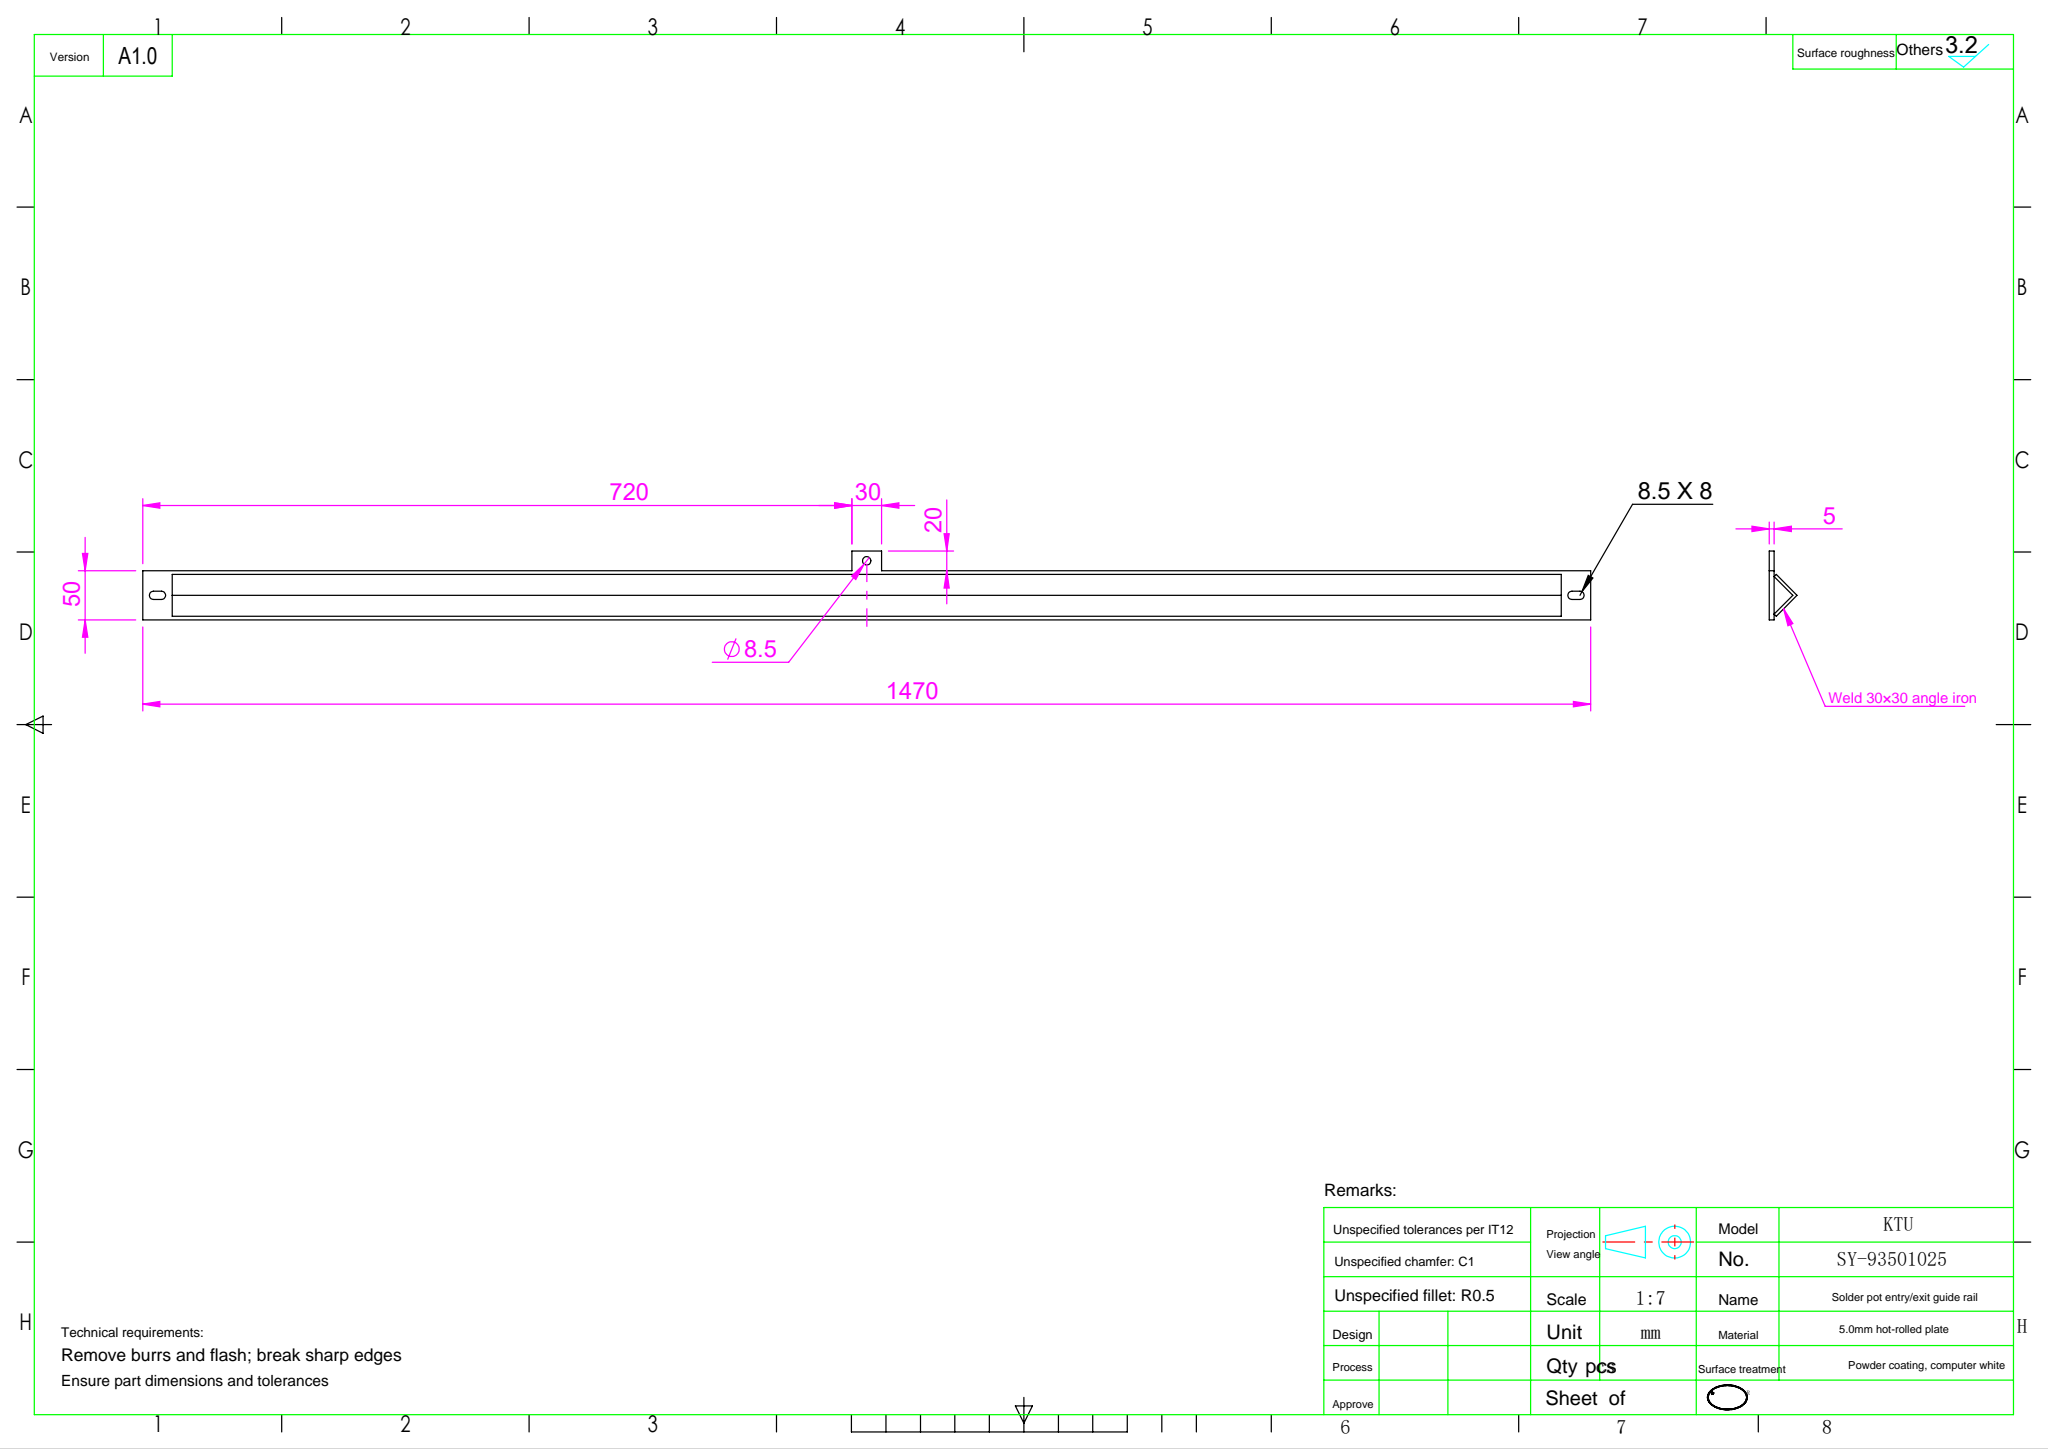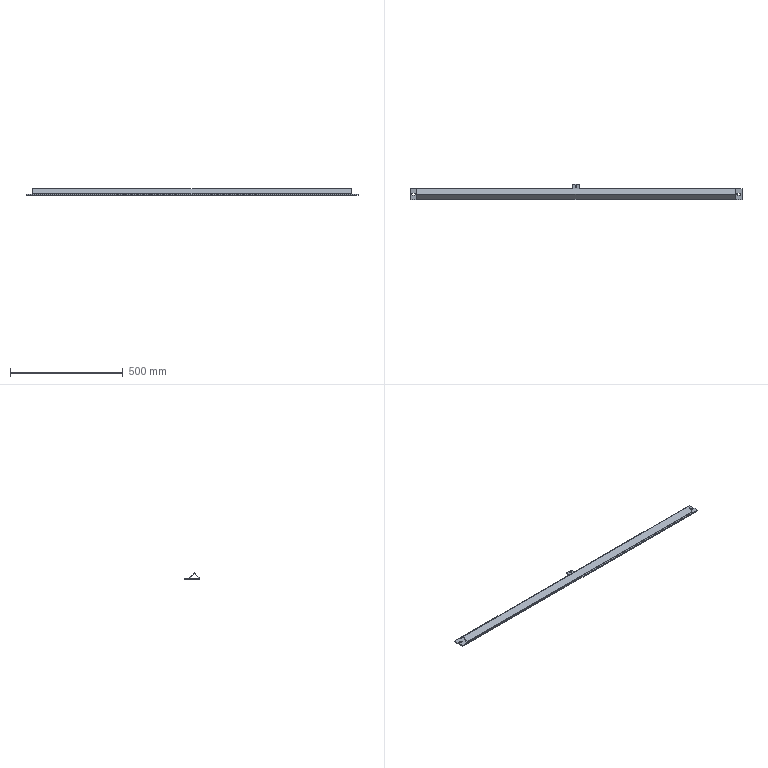Part | SolidWorks | features ICE 4, Extrusion 1 | 2 solids | 30 faces | box 1470 x 70 x 28.335 mm | volume 610079 mm3 | plane 22 | cylinder 8 | commonest cylinder face diameters 8.5 x8
STEP:
#1=CARTESIAN_POINT('',(-705.,21.213,4.621));
#2=VERTEX_POINT('',#1);
#3=CARTESIAN_POINT('',(-705.,19.092,2.5));
#4=VERTEX_POINT('',#3);
#5=CARTESIAN_POINT('',(-705.,21.213,4.621));
#6=DIRECTION('',(0.,-0.7071,-0.7071));
#7=VECTOR('',#6,1000.);
#8=LINE('',#5,#7);
#9=EDGE_CURVE('',#2,#4,#8,.T.);
#10=ORIENTED_EDGE('',*,*,#9,.F.);
#11=CARTESIAN_POINT('',(705.,21.213,4.621));
#12=VERTEX_POINT('',#11);
#13=CARTESIAN_POINT('',(705.,21.213,4.621));
#14=DIRECTION('',(-1.,0.,0.));
#15=VECTOR('',#14,1000.);
#16=LINE('',#13,#15);
#17=EDGE_CURVE('',#12,#2,#16,.T.);
#18=ORIENTED_EDGE('',*,*,#17,.F.);
#19=CARTESIAN_POINT('',(705.,19.092,2.5));
#20=VERTEX_POINT('',#19);
#21=CARTESIAN_POINT('',(705.,21.213,4.621));
#22=DIRECTION('',(0.,-0.7071,-0.7071));
#23=VECTOR('',#22,1000.);
#24=LINE('',#21,#23);
#25=EDGE_CURVE('',#12,#20,#24,.T.);
#26=ORIENTED_EDGE('',*,*,#25,.T.);
#27=CARTESIAN_POINT('',(705.,19.092,2.5));
#28=DIRECTION('',(-1.,0.,0.));
#29=VECTOR('',#28,1000.);
#30=LINE('',#27,#29);
#31=EDGE_CURVE('',#20,#4,#30,.T.);
#32=ORIENTED_EDGE('',*,*,#31,.T.);
#33=EDGE_LOOP('',(#10,#18,#26,#32));
#34=FACE_OUTER_BOUND('',#33,.T.);
#35=CARTESIAN_POINT('',(705.,21.213,4.621));
#36=DIRECTION('',(0.,0.7071,-0.7071));
#37=DIRECTION('',(0.,0.7071,0.7071));
#38=AXIS2_PLACEMENT_3D('',#35,#36,#37);
#39=PLANE('',#38);
#40=ADVANCED_FACE('',(#34),#39,.T.);
#41=CARTESIAN_POINT('',(-705.,0.,25.835));
#42=VERTEX_POINT('',#41);
#43=CARTESIAN_POINT('',(-705.,21.213,4.621));
#44=DIRECTION('',(0.,0.7071,-0.7071));
#45=VECTOR('',#44,1000.);
#46=LINE('',#43,#45);
#47=EDGE_CURVE('',#42,#2,#46,.T.);
#48=ORIENTED_EDGE('',*,*,#47,.F.);
#49=CARTESIAN_POINT('',(705.,0.,25.835));
#50=VERTEX_POINT('',#49);
#51=CARTESIAN_POINT('',(705.,0.,25.835));
#52=DIRECTION('',(-1.,0.,0.));
#53=VECTOR('',#52,1000.);
#54=LINE('',#51,#53);
#55=EDGE_CURVE('',#50,#42,#54,.T.);
#56=ORIENTED_EDGE('',*,*,#55,.F.);
#57=CARTESIAN_POINT('',(705.,21.213,4.621));
#58=DIRECTION('',(0.,0.7071,-0.7071));
#59=VECTOR('',#58,1000.);
#60=LINE('',#57,#59);
#61=EDGE_CURVE('',#50,#12,#60,.T.);
#62=ORIENTED_EDGE('',*,*,#61,.T.);
#63=ORIENTED_EDGE('',*,*,#17,.T.);
#64=EDGE_LOOP('',(#48,#56,#62,#63));
#65=FACE_OUTER_BOUND('',#64,.T.);
#66=CARTESIAN_POINT('',(705.,21.213,4.621));
#67=DIRECTION('',(0.,0.7071,0.7071));
#68=DIRECTION('',(0.,-0.7071,0.7071));
#69=AXIS2_PLACEMENT_3D('',#66,#67,#68);
#70=PLANE('',#69);
#71=ADVANCED_FACE('',(#65),#70,.T.);
#72=CARTESIAN_POINT('',(-705.,-21.213,4.621));
#73=VERTEX_POINT('',#72);
#74=CARTESIAN_POINT('',(-705.,0.,25.835));
#75=DIRECTION('',(0.,0.7071,0.7071));
#76=VECTOR('',#75,1000.);
#77=LINE('',#74,#76);
#78=EDGE_CURVE('',#73,#42,#77,.T.);
#79=ORIENTED_EDGE('',*,*,#78,.F.);
#80=CARTESIAN_POINT('',(705.,-21.213,4.621));
#81=VERTEX_POINT('',#80);
#82=CARTESIAN_POINT('',(705.,-21.213,4.621));
#83=DIRECTION('',(-1.,0.,0.));
#84=VECTOR('',#83,1000.);
#85=LINE('',#82,#84);
#86=EDGE_CURVE('',#81,#73,#85,.T.);
#87=ORIENTED_EDGE('',*,*,#86,.F.);
#88=CARTESIAN_POINT('',(705.,0.,25.835));
#89=DIRECTION('',(0.,0.7071,0.7071));
#90=VECTOR('',#89,1000.);
#91=LINE('',#88,#90);
#92=EDGE_CURVE('',#81,#50,#91,.T.);
#93=ORIENTED_EDGE('',*,*,#92,.T.);
#94=ORIENTED_EDGE('',*,*,#55,.T.);
#95=EDGE_LOOP('',(#79,#87,#93,#94));
#96=FACE_OUTER_BOUND('',#95,.T.);
#97=CARTESIAN_POINT('',(705.,0.,25.835));
#98=DIRECTION('',(0.,-0.7071,0.7071));
#99=DIRECTION('',(0.,-0.7071,-0.7071));
#100=AXIS2_PLACEMENT_3D('',#97,#98,#99);
#101=PLANE('',#100);
#102=ADVANCED_FACE('',(#96),#101,.T.);
#103=CARTESIAN_POINT('',(-705.,-19.092,2.5));
#104=VERTEX_POINT('',#103);
#105=CARTESIAN_POINT('',(-705.,-19.092,2.5));
#106=DIRECTION('',(0.,-0.7071,0.7071));
#107=VECTOR('',#106,1000.);
#108=LINE('',#105,#107);
#109=EDGE_CURVE('',#104,#73,#108,.T.);
#110=ORIENTED_EDGE('',*,*,#109,.F.);
#111=CARTESIAN_POINT('',(705.,-19.092,2.5));
#112=VERTEX_POINT('',#111);
#113=CARTESIAN_POINT('',(705.,-19.092,2.5));
#114=DIRECTION('',(-1.,0.,0.));
#115=VECTOR('',#114,1000.);
#116=LINE('',#113,#115);
#117=EDGE_CURVE('',#112,#104,#116,.T.);
#118=ORIENTED_EDGE('',*,*,#117,.F.);
#119=CARTESIAN_POINT('',(705.,-19.092,2.5));
#120=DIRECTION('',(0.,-0.7071,0.7071));
#121=VECTOR('',#120,1000.);
#122=LINE('',#119,#121);
#123=EDGE_CURVE('',#112,#81,#122,.T.);
#124=ORIENTED_EDGE('',*,*,#123,.T.);
#125=ORIENTED_EDGE('',*,*,#86,.T.);
#126=EDGE_LOOP('',(#110,#118,#124,#125));
#127=FACE_OUTER_BOUND('',#126,.T.);
#128=CARTESIAN_POINT('',(705.,-19.092,2.5));
#129=DIRECTION('',(0.,-0.7071,-0.7071));
#130=DIRECTION('',(0.,0.7071,-0.7071));
#131=AXIS2_PLACEMENT_3D('',#128,#129,#130);
#132=PLANE('',#131);
#133=ADVANCED_FACE('',(#127),#132,.T.);
#134=CARTESIAN_POINT('',(-705.,0.,21.592));
#135=VERTEX_POINT('',#134);
#136=CARTESIAN_POINT('',(-705.,0.,21.592));
#137=DIRECTION('',(0.,-0.7071,-0.7071));
#138=VECTOR('',#137,1000.);
#139=LINE('',#136,#138);
#140=EDGE_CURVE('',#135,#104,#139,.T.);
#141=ORIENTED_EDGE('',*,*,#140,.F.);
#142=CARTESIAN_POINT('',(705.,0.,21.592));
#143=VERTEX_POINT('',#142);
#144=CARTESIAN_POINT('',(705.,0.,21.592));
#145=DIRECTION('',(-1.,0.,0.));
#146=VECTOR('',#145,1000.);
#147=LINE('',#144,#146);
#148=EDGE_CURVE('',#143,#135,#147,.T.);
#149=ORIENTED_EDGE('',*,*,#148,.F.);
#150=CARTESIAN_POINT('',(705.,0.,21.592));
#151=DIRECTION('',(0.,-0.7071,-0.7071));
#152=VECTOR('',#151,1000.);
#153=LINE('',#150,#152);
#154=EDGE_CURVE('',#143,#112,#153,.T.);
#155=ORIENTED_EDGE('',*,*,#154,.T.);
#156=ORIENTED_EDGE('',*,*,#117,.T.);
#157=EDGE_LOOP('',(#141,#149,#155,#156));
#158=FACE_OUTER_BOUND('',#157,.T.);
#159=CARTESIAN_POINT('',(705.,0.,21.592));
#160=DIRECTION('',(0.,0.7071,-0.7071));
#161=DIRECTION('',(0.,0.7071,0.7071));
#162=AXIS2_PLACEMENT_3D('',#159,#160,#161);
#163=PLANE('',#162);
#164=ADVANCED_FACE('',(#158),#163,.T.);
#165=CARTESIAN_POINT('',(-705.,19.092,2.5));
#166=DIRECTION('',(0.,-0.7071,0.7071));
#167=VECTOR('',#166,1000.);
#168=LINE('',#165,#167);
#169=EDGE_CURVE('',#4,#135,#168,.T.);
#170=ORIENTED_EDGE('',*,*,#169,.F.);
#171=ORIENTED_EDGE('',*,*,#31,.F.);
#172=CARTESIAN_POINT('',(705.,19.092,2.5));
#173=DIRECTION('',(0.,-0.7071,0.7071));
#174=VECTOR('',#173,1000.);
#175=LINE('',#172,#174);
#176=EDGE_CURVE('',#20,#143,#175,.T.);
#177=ORIENTED_EDGE('',*,*,#176,.T.);
#178=ORIENTED_EDGE('',*,*,#148,.T.);
#179=EDGE_LOOP('',(#170,#171,#177,#178));
#180=FACE_OUTER_BOUND('',#179,.T.);
#181=CARTESIAN_POINT('',(705.,19.092,2.5));
#182=DIRECTION('',(0.,-0.7071,-0.7071));
#183=DIRECTION('',(0.,0.7071,-0.7071));
#184=AXIS2_PLACEMENT_3D('',#181,#182,#183);
#185=PLANE('',#184);
#186=ADVANCED_FACE('',(#180),#185,.T.);
#187=ORIENTED_EDGE('',*,*,#25,.F.);
#188=ORIENTED_EDGE('',*,*,#61,.F.);
#189=ORIENTED_EDGE('',*,*,#92,.F.);
#190=ORIENTED_EDGE('',*,*,#123,.F.);
#191=ORIENTED_EDGE('',*,*,#154,.F.);
#192=ORIENTED_EDGE('',*,*,#176,.F.);
#193=EDGE_LOOP('',(#187,#188,#189,#190,#191,#192));
#194=FACE_OUTER_BOUND('',#193,.T.);
#195=CARTESIAN_POINT('',(705.,0.,0.));
#196=DIRECTION('',(-1.,0.,0.));
#197=DIRECTION('',(0.,0.,1.));
#198=AXIS2_PLACEMENT_3D('',#195,#196,#197);
#199=PLANE('',#198);
#200=ADVANCED_FACE('',(#194),#199,.F.);
#201=ORIENTED_EDGE('',*,*,#9,.T.);
#202=ORIENTED_EDGE('',*,*,#169,.T.);
#203=ORIENTED_EDGE('',*,*,#140,.T.);
#204=ORIENTED_EDGE('',*,*,#109,.T.);
#205=ORIENTED_EDGE('',*,*,#78,.T.);
#206=ORIENTED_EDGE('',*,*,#47,.T.);
#207=EDGE_LOOP('',(#201,#202,#203,#204,#205,#206));
#208=FACE_OUTER_BOUND('',#207,.T.);
#209=CARTESIAN_POINT('',(-705.,0.,0.));
#210=DIRECTION('',(-1.,0.,0.));
#211=DIRECTION('',(0.,0.,1.));
#212=AXIS2_PLACEMENT_3D('',#209,#210,#211);
#213=PLANE('',#212);
#214=ADVANCED_FACE('',(#208),#213,.T.);
#215=CLOSED_SHELL('',(#40,#71,#102,#133,#164,#186,#200,#214));
#216=MANIFOLD_SOLID_BREP('',#215);
#217=CARTESIAN_POINT('',(4.25,35.,-2.5));
#218=VERTEX_POINT('',#217);
#219=CARTESIAN_POINT('',(-4.25,35.,-2.5));
#220=VERTEX_POINT('',#219);
#221=CARTESIAN_POINT('',(0.,35.,-2.5));
#222=DIRECTION('',(0.,0.,-1.));
#223=DIRECTION('',(1.,0.,0.));
#224=AXIS2_PLACEMENT_3D('',#221,#222,#223);
#225=CIRCLE('',#224,4.25);
#226=EDGE_CURVE('',#218,#220,#225,.T.);
#227=ORIENTED_EDGE('',*,*,#226,.T.);
#228=CARTESIAN_POINT('',(-4.25,35.,2.5));
#229=VERTEX_POINT('',#228);
#230=CARTESIAN_POINT('',(-4.25,35.,-2.501));
#231=DIRECTION('',(0.,0.,1.));
#232=VECTOR('',#231,1000.);
#233=LINE('',#230,#232);
#234=EDGE_CURVE('',#220,#229,#233,.T.);
#235=ORIENTED_EDGE('',*,*,#234,.T.);
#236=CARTESIAN_POINT('',(4.25,35.,2.5));
#237=VERTEX_POINT('',#236);
#238=CARTESIAN_POINT('',(0.,35.,2.5));
#239=DIRECTION('',(0.,0.,1.));
#240=DIRECTION('',(1.,0.,0.));
#241=AXIS2_PLACEMENT_3D('',#238,#239,#240);
#242=CIRCLE('',#241,4.25);
#243=EDGE_CURVE('',#229,#237,#242,.T.);
#244=ORIENTED_EDGE('',*,*,#243,.T.);
#245=CARTESIAN_POINT('',(4.25,35.,-2.501));
#246=DIRECTION('',(0.,0.,1.));
#247=VECTOR('',#246,1000.);
#248=LINE('',#245,#247);
#249=EDGE_CURVE('',#218,#237,#248,.T.);
#250=ORIENTED_EDGE('',*,*,#249,.F.);
#251=EDGE_LOOP('',(#227,#235,#244,#250));
#252=FACE_OUTER_BOUND('',#251,.T.);
#253=CARTESIAN_POINT('',(0.,35.,-2.501));
#254=DIRECTION('',(0.,0.,1.));
#255=DIRECTION('',(1.,0.,0.));
#256=AXIS2_PLACEMENT_3D('',#253,#254,#255);
#257=CYLINDRICAL_SURFACE('',#256,4.25);
#258=ADVANCED_FACE('',(#252),#257,.F.);
#259=CARTESIAN_POINT('',(-716.,4.25,-2.5));
#260=VERTEX_POINT('',#259);
#261=CARTESIAN_POINT('',(-711.75,0.,-2.5));
#262=VERTEX_POINT('',#261);
#263=CARTESIAN_POINT('',(-716.,0.,-2.5));
#264=DIRECTION('',(0.,0.,-1.));
#265=DIRECTION('',(1.,0.,0.));
#266=AXIS2_PLACEMENT_3D('',#263,#264,#265);
#267=CIRCLE('',#266,4.25);
#268=EDGE_CURVE('',#260,#262,#267,.T.);
#269=ORIENTED_EDGE('',*,*,#268,.T.);
#270=CARTESIAN_POINT('',(-711.75,0.,2.5));
#271=VERTEX_POINT('',#270);
#272=CARTESIAN_POINT('',(-711.75,0.,-2.501));
#273=DIRECTION('',(0.,0.,1.));
#274=VECTOR('',#273,1000.);
#275=LINE('',#272,#274);
#276=EDGE_CURVE('',#262,#271,#275,.T.);
#277=ORIENTED_EDGE('',*,*,#276,.T.);
#278=CARTESIAN_POINT('',(-716.,4.25,2.5));
#279=VERTEX_POINT('',#278);
#280=CARTESIAN_POINT('',(-716.,0.,2.5));
#281=DIRECTION('',(0.,0.,1.));
#282=DIRECTION('',(1.,0.,0.));
#283=AXIS2_PLACEMENT_3D('',#280,#281,#282);
#284=CIRCLE('',#283,4.25);
#285=EDGE_CURVE('',#271,#279,#284,.T.);
#286=ORIENTED_EDGE('',*,*,#285,.T.);
#287=CARTESIAN_POINT('',(-716.,4.25,-2.501));
#288=DIRECTION('',(0.,0.,1.));
#289=VECTOR('',#288,1000.);
#290=LINE('',#287,#289);
#291=EDGE_CURVE('',#260,#279,#290,.T.);
#292=ORIENTED_EDGE('',*,*,#291,.F.);
#293=EDGE_LOOP('',(#269,#277,#286,#292));
#294=FACE_OUTER_BOUND('',#293,.T.);
#295=CARTESIAN_POINT('',(-716.,0.,-2.501));
#296=DIRECTION('',(0.,0.,1.));
#297=DIRECTION('',(1.,0.,0.));
#298=AXIS2_PLACEMENT_3D('',#295,#296,#297);
#299=CYLINDRICAL_SURFACE('',#298,4.25);
#300=ADVANCED_FACE('',(#294),#299,.F.);
#301=CARTESIAN_POINT('',(724.,4.25,-2.5));
#302=VERTEX_POINT('',#301);
#303=CARTESIAN_POINT('',(728.25,0.,-2.5));
#304=VERTEX_POINT('',#303);
#305=CARTESIAN_POINT('',(724.,0.,-2.5));
#306=DIRECTION('',(0.,0.,-1.));
#307=DIRECTION('',(1.,0.,0.));
#308=AXIS2_PLACEMENT_3D('',#305,#306,#307);
#309=CIRCLE('',#308,4.25);
#310=EDGE_CURVE('',#302,#304,#309,.T.);
#311=ORIENTED_EDGE('',*,*,#310,.T.);
#312=CARTESIAN_POINT('',(728.25,0.,2.5));
#313=VERTEX_POINT('',#312);
#314=CARTESIAN_POINT('',(728.25,0.,-2.501));
#315=DIRECTION('',(0.,0.,1.));
#316=VECTOR('',#315,1000.);
#317=LINE('',#314,#316);
#318=EDGE_CURVE('',#304,#313,#317,.T.);
#319=ORIENTED_EDGE('',*,*,#318,.T.);
#320=CARTESIAN_POINT('',(724.,4.25,2.5));
#321=VERTEX_POINT('',#320);
#322=CARTESIAN_POINT('',(724.,0.,2.5));
#323=DIRECTION('',(0.,0.,1.));
#324=DIRECTION('',(1.,0.,0.));
#325=AXIS2_PLACEMENT_3D('',#322,#323,#324);
#326=CIRCLE('',#325,4.25);
#327=EDGE_CURVE('',#313,#321,#326,.T.);
#328=ORIENTED_EDGE('',*,*,#327,.T.);
#329=CARTESIAN_POINT('',(724.,4.25,-2.501));
#330=DIRECTION('',(0.,0.,1.));
#331=VECTOR('',#330,1000.);
#332=LINE('',#329,#331);
#333=EDGE_CURVE('',#302,#321,#332,.T.);
#334=ORIENTED_EDGE('',*,*,#333,.F.);
#335=EDGE_LOOP('',(#311,#319,#328,#334));
#336=FACE_OUTER_BOUND('',#335,.T.);
#337=CARTESIAN_POINT('',(724.,0.,-2.501));
#338=DIRECTION('',(0.,0.,1.));
#339=DIRECTION('',(1.,0.,0.));
#340=AXIS2_PLACEMENT_3D('',#337,#338,#339);
#341=CYLINDRICAL_SURFACE('',#340,4.25);
#342=ADVANCED_FACE('',(#336),#341,.F.);
#343=CARTESIAN_POINT('',(-15.,25.,-2.5));
#344=VERTEX_POINT('',#343);
#345=CARTESIAN_POINT('',(-15.,25.,2.5));
#346=VERTEX_POINT('',#345);
#347=CARTESIAN_POINT('',(-15.,25.,-2.5));
#348=DIRECTION('',(0.,0.,1.));
#349=VECTOR('',#348,1000.);
#350=LINE('',#347,#349);
#351=EDGE_CURVE('',#344,#346,#350,.T.);
#352=ORIENTED_EDGE('',*,*,#351,.F.);
#353=CARTESIAN_POINT('',(-735.,25.,-2.5));
#354=VERTEX_POINT('',#353);
#355=CARTESIAN_POINT('',(-735.,25.,-2.5));
#356=DIRECTION('',(-1.,0.,0.));
#357=VECTOR('',#356,1000.);
#358=LINE('',#355,#357);
#359=EDGE_CURVE('',#344,#354,#358,.T.);
#360=ORIENTED_EDGE('',*,*,#359,.T.);
#361=CARTESIAN_POINT('',(-735.,25.,2.5));
#362=VERTEX_POINT('',#361);
#363=CARTESIAN_POINT('',(-735.,25.,2.5));
#364=DIRECTION('',(0.,0.,-1.));
#365=VECTOR('',#364,1000.);
#366=LINE('',#363,#365);
#367=EDGE_CURVE('',#362,#354,#366,.T.);
#368=ORIENTED_EDGE('',*,*,#367,.F.);
#369=CARTESIAN_POINT('',(-735.,25.,2.5));
#370=DIRECTION('',(-1.,0.,0.));
#371=VECTOR('',#370,1000.);
#372=LINE('',#369,#371);
#373=EDGE_CURVE('',#346,#362,#372,.T.);
#374=ORIENTED_EDGE('',*,*,#373,.F.);
#375=EDGE_LOOP('',(#352,#360,#368,#374));
#376=FACE_OUTER_BOUND('',#375,.T.);
#377=CARTESIAN_POINT('',(-735.,25.,2.5));
#378=DIRECTION('',(0.,-1.,0.));
#379=DIRECTION('',(0.,0.,-1.));
#380=AXIS2_PLACEMENT_3D('',#377,#378,#379);
#381=PLANE('',#380);
#382=ADVANCED_FACE('',(#376),#381,.F.);
#383=CARTESIAN_POINT('',(735.,-25.,-2.5));
#384=VERTEX_POINT('',#383);
#385=CARTESIAN_POINT('',(735.,25.,-2.5));
#386=VERTEX_POINT('',#385);
#387=CARTESIAN_POINT('',(735.,25.,-2.5));
#388=DIRECTION('',(0.,1.,0.));
#389=VECTOR('',#388,1000.);
#390=LINE('',#387,#389);
#391=EDGE_CURVE('',#384,#386,#390,.T.);
#392=ORIENTED_EDGE('',*,*,#391,.T.);
#393=CARTESIAN_POINT('',(735.,25.,2.5));
#394=VERTEX_POINT('',#393);
#395=CARTESIAN_POINT('',(735.,25.,2.5));
#396=DIRECTION('',(0.,0.,-1.));
#397=VECTOR('',#396,1000.);
#398=LINE('',#395,#397);
#399=EDGE_CURVE('',#394,#386,#398,.T.);
#400=ORIENTED_EDGE('',*,*,#399,.F.);
#401=CARTESIAN_POINT('',(735.,-25.,2.5));
#402=VERTEX_POINT('',#401);
#403=CARTESIAN_POINT('',(735.,25.,2.5));
#404=DIRECTION('',(0.,1.,0.));
#405=VECTOR('',#404,1000.);
#406=LINE('',#403,#405);
#407=EDGE_CURVE('',#402,#394,#406,.T.);
#408=ORIENTED_EDGE('',*,*,#407,.F.);
#409=CARTESIAN_POINT('',(735.,-25.,2.5));
#410=DIRECTION('',(0.,0.,-1.));
#411=VECTOR('',#410,1000.);
#412=LINE('',#409,#411);
#413=EDGE_CURVE('',#402,#384,#412,.T.);
#414=ORIENTED_EDGE('',*,*,#413,.T.);
#415=EDGE_LOOP('',(#392,#400,#408,#414));
#416=FACE_OUTER_BOUND('',#415,.T.);
#417=CARTESIAN_POINT('',(735.,25.,2.5));
#418=DIRECTION('',(-1.,0.,0.));
#419=DIRECTION('',(0.,0.,1.));
#420=AXIS2_PLACEMENT_3D('',#417,#418,#419);
#421=PLANE('',#420);
#422=ADVANCED_FACE('',(#416),#421,.F.);
#423=CARTESIAN_POINT('',(15.,25.,-2.5));
#424=VERTEX_POINT('',#423);
#425=CARTESIAN_POINT('',(-735.,25.,-2.5));
#426=DIRECTION('',(-1.,0.,0.));
#427=VECTOR('',#426,1000.);
#428=LINE('',#425,#427);
#429=EDGE_CURVE('',#386,#424,#428,.T.);
#430=ORIENTED_EDGE('',*,*,#429,.T.);
#431=CARTESIAN_POINT('',(15.,25.,2.5));
#432=VERTEX_POINT('',#431);
#433=CARTESIAN_POINT('',(15.,25.,-2.5));
#434=DIRECTION('',(0.,0.,1.));
#435=VECTOR('',#434,1000.);
#436=LINE('',#433,#435);
#437=EDGE_CURVE('',#424,#432,#436,.T.);
#438=ORIENTED_EDGE('',*,*,#437,.T.);
#439=CARTESIAN_POINT('',(-735.,25.,2.5));
#440=DIRECTION('',(-1.,0.,0.));
#441=VECTOR('',#440,1000.);
#442=LINE('',#439,#441);
#443=EDGE_CURVE('',#394,#432,#442,.T.);
#444=ORIENTED_EDGE('',*,*,#443,.F.);
#445=ORIENTED_EDGE('',*,*,#399,.T.);
#446=EDGE_LOOP('',(#430,#438,#444,#445));
#447=FACE_OUTER_BOUND('',#446,.T.);
#448=CARTESIAN_POINT('',(-735.,25.,2.5));
#449=DIRECTION('',(0.,-1.,0.));
#450=DIRECTION('',(0.,0.,-1.));
#451=AXIS2_PLACEMENT_3D('',#448,#449,#450);
#452=PLANE('',#451);
#453=ADVANCED_FACE('',(#447),#452,.F.);
#454=CARTESIAN_POINT('',(-735.,-25.,-2.5));
#455=VERTEX_POINT('',#454);
#456=CARTESIAN_POINT('',(-735.,25.,-2.5));
#457=DIRECTION('',(0.,-1.,0.));
#458=VECTOR('',#457,1000.);
#459=LINE('',#456,#458);
#460=EDGE_CURVE('',#354,#455,#459,.T.);
#461=ORIENTED_EDGE('',*,*,#460,.T.);
#462=CARTESIAN_POINT('',(-735.,-25.,2.5));
#463=VERTEX_POINT('',#462);
#464=CARTESIAN_POINT('',(-735.,-25.,2.5));
#465=DIRECTION('',(0.,0.,-1.));
#466=VECTOR('',#465,1000.);
#467=LINE('',#464,#466);
#468=EDGE_CURVE('',#463,#455,#467,.T.);
#469=ORIENTED_EDGE('',*,*,#468,.F.);
#470=CARTESIAN_POINT('',(-735.,25.,2.5));
#471=DIRECTION('',(0.,-1.,0.));
#472=VECTOR('',#471,1000.);
#473=LINE('',#470,#472);
#474=EDGE_CURVE('',#362,#463,#473,.T.);
#475=ORIENTED_EDGE('',*,*,#474,.F.);
#476=ORIENTED_EDGE('',*,*,#367,.T.);
#477=EDGE_LOOP('',(#461,#469,#475,#476));
#478=FACE_OUTER_BOUND('',#477,.T.);
#479=CARTESIAN_POINT('',(-735.,25.,2.5));
#480=DIRECTION('',(1.,0.,0.));
#481=DIRECTION('',(0.,0.,-1.));
#482=AXIS2_PLACEMENT_3D('',#479,#480,#481);
#483=PLANE('',#482);
#484=ADVANCED_FACE('',(#478),#483,.F.);
#485=CARTESIAN_POINT('',(-735.,-25.,-2.5));
#486=DIRECTION('',(1.,0.,0.));
#487=VECTOR('',#486,1000.);
#488=LINE('',#485,#487);
#489=EDGE_CURVE('',#455,#384,#488,.T.);
#490=ORIENTED_EDGE('',*,*,#489,.T.);
#491=ORIENTED_EDGE('',*,*,#413,.F.);
#492=CARTESIAN_POINT('',(-735.,-25.,2.5));
#493=DIRECTION('',(1.,0.,0.));
#494=VECTOR('',#493,1000.);
#495=LINE('',#492,#494);
#496=EDGE_CURVE('',#463,#402,#495,.T.);
#497=ORIENTED_EDGE('',*,*,#496,.F.);
#498=ORIENTED_EDGE('',*,*,#468,.T.);
#499=EDGE_LOOP('',(#490,#491,#497,#498));
#500=FACE_OUTER_BOUND('',#499,.T.);
#501=CARTESIAN_POINT('',(-735.,-25.,2.5));
#502=DIRECTION('',(0.,1.,0.));
#503=DIRECTION('',(0.,0.,1.));
#504=AXIS2_PLACEMENT_3D('',#501,#502,#503);
#505=PLANE('',#504);
#506=ADVANCED_FACE('',(#500),#505,.F.);
#507=CARTESIAN_POINT('',(0.,35.,2.5));
#508=DIRECTION('',(0.,0.,1.));
#509=DIRECTION('',(1.,0.,0.));
#510=AXIS2_PLACEMENT_3D('',#507,#508,#509);
#511=CIRCLE('',#510,4.25);
#512=EDGE_CURVE('',#237,#229,#511,.T.);
#513=ORIENTED_EDGE('',*,*,#512,.F.);
#514=ORIENTED_EDGE('',*,*,#243,.F.);
#515=EDGE_LOOP('',(#513,#514));
#516=FACE_BOUND('',#515,.T.);
#517=CARTESIAN_POINT('',(-716.,-4.25,2.5));
#518=VERTEX_POINT('',#517);
#519=CARTESIAN_POINT('',(-716.,0.,2.5));
#520=DIRECTION('',(0.,0.,1.));
#521=DIRECTION('',(1.,0.,0.));
#522=AXIS2_PLACEMENT_3D('',#519,#520,#521);
#523=CIRCLE('',#522,4.25);
#524=EDGE_CURVE('',#518,#271,#523,.T.);
#525=ORIENTED_EDGE('',*,*,#524,.F.);
#526=CARTESIAN_POINT('',(-724.,-4.25,2.5));
#527=VERTEX_POINT('',#526);
#528=CARTESIAN_POINT('',(-716.,-4.25,2.5));
#529=DIRECTION('',(1.,0.,0.));
#530=VECTOR('',#529,1000.);
#531=LINE('',#528,#530);
#532=EDGE_CURVE('',#527,#518,#531,.T.);
#533=ORIENTED_EDGE('',*,*,#532,.F.);
#534=CARTESIAN_POINT('',(-724.,4.25,2.5));
#535=VERTEX_POINT('',#534);
#536=CARTESIAN_POINT('',(-724.,0.,2.5));
#537=DIRECTION('',(0.,0.,1.));
#538=DIRECTION('',(1.,0.,0.));
#539=AXIS2_PLACEMENT_3D('',#536,#537,#538);
#540=CIRCLE('',#539,4.25);
#541=EDGE_CURVE('',#535,#527,#540,.T.);
#542=ORIENTED_EDGE('',*,*,#541,.F.);
#543=CARTESIAN_POINT('',(-716.,4.25,2.5));
#544=DIRECTION('',(-1.,0.,0.));
#545=VECTOR('',#544,1000.);
#546=LINE('',#543,#545);
#547=EDGE_CURVE('',#279,#535,#546,.T.);
#548=ORIENTED_EDGE('',*,*,#547,.F.);
#549=ORIENTED_EDGE('',*,*,#285,.F.);
#550=EDGE_LOOP('',(#525,#533,#542,#548,#549));
#551=FACE_BOUND('',#550,.T.);
#552=CARTESIAN_POINT('',(716.,4.25,2.5));
#553=VERTEX_POINT('',#552);
#554=CARTESIAN_POINT('',(716.,-4.25,2.5));
#555=VERTEX_POINT('',#554);
#556=CARTESIAN_POINT('',(716.,0.,2.5));
#557=DIRECTION('',(0.,0.,1.));
#558=DIRECTION('',(1.,0.,0.));
#559=AXIS2_PLACEMENT_3D('',#556,#557,#558);
#560=CIRCLE('',#559,4.25);
#561=EDGE_CURVE('',#553,#555,#560,.T.);
#562=ORIENTED_EDGE('',*,*,#561,.F.);
#563=CARTESIAN_POINT('',(716.,4.25,2.5));
#564=DIRECTION('',(-1.,0.,0.));
#565=VECTOR('',#564,1000.);
#566=LINE('',#563,#565);
#567=EDGE_CURVE('',#321,#553,#566,.T.);
#568=ORIENTED_EDGE('',*,*,#567,.F.);
#569=ORIENTED_EDGE('',*,*,#327,.F.);
#570=CARTESIAN_POINT('',(724.,-4.25,2.5));
#571=VERTEX_POINT('',#570);
#572=CARTESIAN_POINT('',(724.,0.,2.5));
#573=DIRECTION('',(0.,0.,1.));
#574=DIRECTION('',(1.,0.,0.));
#575=AXIS2_PLACEMENT_3D('',#572,#573,#574);
#576=CIRCLE('',#575,4.25);
#577=EDGE_CURVE('',#571,#313,#576,.T.);
#578=ORIENTED_EDGE('',*,*,#577,.F.);
#579=CARTESIAN_POINT('',(716.,-4.25,2.5));
#580=DIRECTION('',(1.,0.,0.));
#581=VECTOR('',#580,1000.);
#582=LINE('',#579,#581);
#583=EDGE_CURVE('',#555,#571,#582,.T.);
#584=ORIENTED_EDGE('',*,*,#583,.F.);
#585=EDGE_LOOP('',(#562,#568,#569,#578,#584));
#586=FACE_BOUND('',#585,.T.);
#587=ORIENTED_EDGE('',*,*,#407,.T.);
#588=ORIENTED_EDGE('',*,*,#443,.T.);
#589=CARTESIAN_POINT('',(15.,45.,2.5));
#590=VERTEX_POINT('',#589);
#591=CARTESIAN_POINT('',(15.,25.,2.5));
#592=DIRECTION('',(0.,1.,0.));
#593=VECTOR('',#592,1000.);
#594=LINE('',#591,#593);
#595=EDGE_CURVE('',#432,#590,#594,.T.);
#596=ORIENTED_EDGE('',*,*,#595,.T.);
#597=CARTESIAN_POINT('',(-15.,45.,2.5));
#598=VERTEX_POINT('',#597);
#599=CARTESIAN_POINT('',(15.,45.,2.5));
#600=DIRECTION('',(-1.,0.,0.));
#601=VECTOR('',#600,1000.);
#602=LINE('',#599,#601);
#603=EDGE_CURVE('',#590,#598,#602,.T.);
#604=ORIENTED_EDGE('',*,*,#603,.T.);
#605=CARTESIAN_POINT('',(-15.,25.,2.5));
#606=DIRECTION('',(0.,-1.,0.));
#607=VECTOR('',#606,1000.);
#608=LINE('',#605,#607);
#609=EDGE_CURVE('',#598,#346,#608,.T.);
#610=ORIENTED_EDGE('',*,*,#609,.T.);
#611=ORIENTED_EDGE('',*,*,#373,.T.);
#612=ORIENTED_EDGE('',*,*,#474,.T.);
#613=ORIENTED_EDGE('',*,*,#496,.T.);
#614=EDGE_LOOP('',(#587,#588,#596,#604,#610,#611,#612,#613));
#615=FACE_OUTER_BOUND('',#614,.T.);
#616=CARTESIAN_POINT('',(0.,0.,2.5));
#617=DIRECTION('',(0.,0.,1.));
#618=DIRECTION('',(1.,0.,0.));
#619=AXIS2_PLACEMENT_3D('',#616,#617,#618);
#620=PLANE('',#619);
#621=ADVANCED_FACE('',(#516,#551,#586,#615),#620,.T.);
#622=ORIENTED_EDGE('',*,*,#226,.F.);
#623=CARTESIAN_POINT('',(0.,35.,-2.5));
#624=DIRECTION('',(0.,0.,-1.));
#625=DIRECTION('',(1.,0.,0.));
#626=AXIS2_PLACEMENT_3D('',#623,#624,#625);
#627=CIRCLE('',#626,4.25);
#628=EDGE_CURVE('',#220,#218,#627,.T.);
#629=ORIENTED_EDGE('',*,*,#628,.F.);
#630=EDGE_LOOP('',(#622,#629));
#631=FACE_BOUND('',#630,.T.);
#632=CARTESIAN_POINT('',(-716.,-4.25,-2.5));
#633=VERTEX_POINT('',#632);
#634=CARTESIAN_POINT('',(-724.,-4.25,-2.5));
#635=VERTEX_POINT('',#634);
#636=CARTESIAN_POINT('',(-716.,-4.25,-2.5));
#637=DIRECTION('',(-1.,0.,0.));
#638=VECTOR('',#637,1000.);
#639=LINE('',#636,#638);
#640=EDGE_CURVE('',#633,#635,#639,.T.);
#641=ORIENTED_EDGE('',*,*,#640,.F.);
#642=CARTESIAN_POINT('',(-716.,0.,-2.5));
#643=DIRECTION('',(0.,0.,-1.));
#644=DIRECTION('',(1.,0.,0.));
#645=AXIS2_PLACEMENT_3D('',#642,#643,#644);
#646=CIRCLE('',#645,4.25);
#647=EDGE_CURVE('',#262,#633,#646,.T.);
#648=ORIENTED_EDGE('',*,*,#647,.F.);
#649=ORIENTED_EDGE('',*,*,#268,.F.);
#650=CARTESIAN_POINT('',(-724.,4.25,-2.5));
#651=VERTEX_POINT('',#650);
#652=CARTESIAN_POINT('',(-716.,4.25,-2.5));
#653=DIRECTION('',(1.,0.,0.));
#654=VECTOR('',#653,1000.);
#655=LINE('',#652,#654);
#656=EDGE_CURVE('',#651,#260,#655,.T.);
#657=ORIENTED_EDGE('',*,*,#656,.F.);
#658=CARTESIAN_POINT('',(-724.,0.,-2.5));
#659=DIRECTION('',(0.,0.,-1.));
#660=DIRECTION('',(1.,0.,0.));
#661=AXIS2_PLACEMENT_3D('',#658,#659,#660);
#662=CIRCLE('',#661,4.25);
#663=EDGE_CURVE('',#635,#651,#662,.T.);
#664=ORIENTED_EDGE('',*,*,#663,.F.);
#665=EDGE_LOOP('',(#641,#648,#649,#657,#664));
#666=FACE_BOUND('',#665,.T.);
#667=CARTESIAN_POINT('',(716.,4.25,-2.5));
#668=VERTEX_POINT('',#667);
#669=CARTESIAN_POINT('',(716.,4.25,-2.5));
#670=DIRECTION('',(1.,0.,0.));
#671=VECTOR('',#670,1000.);
#672=LINE('',#669,#671);
#673=EDGE_CURVE('',#668,#302,#672,.T.);
#674=ORIENTED_EDGE('',*,*,#673,.F.);
#675=CARTESIAN_POINT('',(716.,-4.25,-2.5));
#676=VERTEX_POINT('',#675);
#677=CARTESIAN_POINT('',(716.,0.,-2.5));
#678=DIRECTION('',(0.,0.,-1.));
#679=DIRECTION('',(1.,0.,0.));
#680=AXIS2_PLACEMENT_3D('',#677,#678,#679);
#681=CIRCLE('',#680,4.25);
#682=EDGE_CURVE('',#676,#668,#681,.T.);
#683=ORIENTED_EDGE('',*,*,#682,.F.);
#684=CARTESIAN_POINT('',(724.,-4.25,-2.5));
#685=VERTEX_POINT('',#684);
#686=CARTESIAN_POINT('',(716.,-4.25,-2.5));
#687=DIRECTION('',(-1.,0.,0.));
#688=VECTOR('',#687,1000.);
#689=LINE('',#686,#688);
#690=EDGE_CURVE('',#685,#676,#689,.T.);
#691=ORIENTED_EDGE('',*,*,#690,.F.);
#692=CARTESIAN_POINT('',(724.,0.,-2.5));
#693=DIRECTION('',(0.,0.,-1.));
#694=DIRECTION('',(1.,0.,0.));
#695=AXIS2_PLACEMENT_3D('',#692,#693,#694);
#696=CIRCLE('',#695,4.25);
#697=EDGE_CURVE('',#304,#685,#696,.T.);
#698=ORIENTED_EDGE('',*,*,#697,.F.);
#699=ORIENTED_EDGE('',*,*,#310,.F.);
#700=EDGE_LOOP('',(#674,#683,#691,#698,#699));
#701=FACE_BOUND('',#700,.T.);
#702=ORIENTED_EDGE('',*,*,#391,.F.);
#703=ORIENTED_EDGE('',*,*,#489,.F.);
#704=ORIENTED_EDGE('',*,*,#460,.F.);
#705=ORIENTED_EDGE('',*,*,#359,.F.);
#706=CARTESIAN_POINT('',(-15.,45.,-2.5));
#707=VERTEX_POINT('',#706);
#708=CARTESIAN_POINT('',(-15.,25.,-2.5));
#709=DIRECTION('',(0.,-1.,0.));
#710=VECTOR('',#709,1000.);
#711=LINE('',#708,#710);
#712=EDGE_CURVE('',#707,#344,#711,.T.);
#713=ORIENTED_EDGE('',*,*,#712,.F.);
#714=CARTESIAN_POINT('',(15.,45.,-2.5));
#715=VERTEX_POINT('',#714);
#716=CARTESIAN_POINT('',(15.,45.,-2.5));
#717=DIRECTION('',(-1.,0.,0.));
#718=VECTOR('',#717,1000.);
#719=LINE('',#716,#718);
#720=EDGE_CURVE('',#715,#707,#719,.T.);
#721=ORIENTED_EDGE('',*,*,#720,.F.);
#722=CARTESIAN_POINT('',(15.,25.,-2.5));
#723=DIRECTION('',(0.,1.,0.));
#724=VECTOR('',#723,1000.);
#725=LINE('',#722,#724);
#726=EDGE_CURVE('',#424,#715,#725,.T.);
#727=ORIENTED_EDGE('',*,*,#726,.F.);
#728=ORIENTED_EDGE('',*,*,#429,.F.);
#729=EDGE_LOOP('',(#702,#703,#704,#705,#713,#721,#727,#728));
#730=FACE_OUTER_BOUND('',#729,.T.);
#731=CARTESIAN_POINT('',(0.,0.,-2.5));
#732=DIRECTION('',(0.,0.,1.));
#733=DIRECTION('',(1.,0.,0.));
#734=AXIS2_PLACEMENT_3D('',#731,#732,#733);
#735=PLANE('',#734);
#736=ADVANCED_FACE('',(#631,#666,#701,#730),#735,.F.);
#737=ORIENTED_EDGE('',*,*,#682,.T.);
#738=CARTESIAN_POINT('',(716.,4.25,-2.501));
#739=DIRECTION('',(0.,0.,1.));
#740=VECTOR('',#739,1000.);
#741=LINE('',#738,#740);
#742=EDGE_CURVE('',#668,#553,#741,.T.);
#743=ORIENTED_EDGE('',*,*,#742,.T.);
#744=ORIENTED_EDGE('',*,*,#561,.T.);
#745=CARTESIAN_POINT('',(716.,-4.25,-2.501));
#746=DIRECTION('',(0.,0.,1.));
#747=VECTOR('',#746,1000.);
#748=LINE('',#745,#747);
#749=EDGE_CURVE('',#676,#555,#748,.T.);
#750=ORIENTED_EDGE('',*,*,#749,.F.);
#751=EDGE_LOOP('',(#737,#743,#744,#750));
#752=FACE_OUTER_BOUND('',#751,.T.);
#753=CARTESIAN_POINT('',(716.,0.,-2.501));
#754=DIRECTION('',(0.,0.,1.));
#755=DIRECTION('',(1.,0.,0.));
#756=AXIS2_PLACEMENT_3D('',#753,#754,#755);
#757=CYLINDRICAL_SURFACE('',#756,4.25);
#758=ADVANCED_FACE('',(#752),#757,.F.);
#759=ORIENTED_EDGE('',*,*,#673,.T.);
#760=ORIENTED_EDGE('',*,*,#333,.T.);
#761=ORIENTED_EDGE('',*,*,#567,.T.);
#762=ORIENTED_EDGE('',*,*,#742,.F.);
#763=EDGE_LOOP('',(#759,#760,#761,#762));
#764=FACE_OUTER_BOUND('',#763,.T.);
#765=CARTESIAN_POINT('',(716.,4.25,-2.501));
#766=DIRECTION('',(0.,1.,0.));
#767=DIRECTION('',(-1.,0.,0.));
#768=AXIS2_PLACEMENT_3D('',#765,#766,#767);
#769=PLANE('',#768);
#770=ADVANCED_FACE('',(#764),#769,.F.);
#771=ORIENTED_EDGE('',*,*,#318,.F.);
#772=ORIENTED_EDGE('',*,*,#697,.T.);
#773=CARTESIAN_POINT('',(724.,-4.25,-2.501));
#774=DIRECTION('',(0.,0.,1.));
#775=VECTOR('',#774,1000.);
#776=LINE('',#773,#775);
#777=EDGE_CURVE('',#685,#571,#776,.T.);
#778=ORIENTED_EDGE('',*,*,#777,.T.);
#779=ORIENTED_EDGE('',*,*,#577,.T.);
#780=EDGE_LOOP('',(#771,#772,#778,#779));
#781=FACE_OUTER_BOUND('',#780,.T.);
#782=CARTESIAN_POINT('',(724.,0.,-2.501));
#783=DIRECTION('',(0.,0.,1.));
#784=DIRECTION('',(1.,0.,0.));
#785=AXIS2_PLACEMENT_3D('',#782,#783,#784);
#786=CYLINDRICAL_SURFACE('',#785,4.25);
#787=ADVANCED_FACE('',(#781),#786,.F.);
#788=ORIENTED_EDGE('',*,*,#690,.T.);
#789=ORIENTED_EDGE('',*,*,#749,.T.);
#790=ORIENTED_EDGE('',*,*,#583,.T.);
#791=ORIENTED_EDGE('',*,*,#777,.F.);
#792=EDGE_LOOP('',(#788,#789,#790,#791));
#793=FACE_OUTER_BOUND('',#792,.T.);
#794=CARTESIAN_POINT('',(716.,-4.25,-2.501));
#795=DIRECTION('',(0.,-1.,0.));
#796=DIRECTION('',(1.,0.,0.));
#797=AXIS2_PLACEMENT_3D('',#794,#795,#796);
#798=PLANE('',#797);
#799=ADVANCED_FACE('',(#793),#798,.F.);
#800=ORIENTED_EDGE('',*,*,#276,.F.);
#801=ORIENTED_EDGE('',*,*,#647,.T.);
#802=CARTESIAN_POINT('',(-716.,-4.25,-2.501));
#803=DIRECTION('',(0.,0.,1.));
#804=VECTOR('',#803,1000.);
#805=LINE('',#802,#804);
#806=EDGE_CURVE('',#633,#518,#805,.T.);
#807=ORIENTED_EDGE('',*,*,#806,.T.);
#808=ORIENTED_EDGE('',*,*,#524,.T.);
#809=EDGE_LOOP('',(#800,#801,#807,#808));
#810=FACE_OUTER_BOUND('',#809,.T.);
#811=CARTESIAN_POINT('',(-716.,0.,-2.501));
#812=DIRECTION('',(0.,0.,1.));
#813=DIRECTION('',(1.,0.,0.));
#814=AXIS2_PLACEMENT_3D('',#811,#812,#813);
#815=CYLINDRICAL_SURFACE('',#814,4.25);
#816=ADVANCED_FACE('',(#810),#815,.F.);
#817=ORIENTED_EDGE('',*,*,#640,.T.);
#818=CARTESIAN_POINT('',(-724.,-4.25,-2.501));
#819=DIRECTION('',(0.,0.,1.));
#820=VECTOR('',#819,1000.);
#821=LINE('',#818,#820);
#822=EDGE_CURVE('',#635,#527,#821,.T.);
#823=ORIENTED_EDGE('',*,*,#822,.T.);
#824=ORIENTED_EDGE('',*,*,#532,.T.);
#825=ORIENTED_EDGE('',*,*,#806,.F.);
#826=EDGE_LOOP('',(#817,#823,#824,#825));
#827=FACE_OUTER_BOUND('',#826,.T.);
#828=CARTESIAN_POINT('',(-716.,-4.25,-2.501));
#829=DIRECTION('',(0.,-1.,0.));
#830=DIRECTION('',(1.,0.,0.));
#831=AXIS2_PLACEMENT_3D('',#828,#829,#830);
#832=PLANE('',#831);
#833=ADVANCED_FACE('',(#827),#832,.F.);
#834=ORIENTED_EDGE('',*,*,#663,.T.);
#835=CARTESIAN_POINT('',(-724.,4.25,-2.501));
#836=DIRECTION('',(0.,0.,1.));
#837=VECTOR('',#836,1000.);
#838=LINE('',#835,#837);
#839=EDGE_CURVE('',#651,#535,#838,.T.);
#840=ORIENTED_EDGE('',*,*,#839,.T.);
#841=ORIENTED_EDGE('',*,*,#541,.T.);
#842=ORIENTED_EDGE('',*,*,#822,.F.);
#843=EDGE_LOOP('',(#834,#840,#841,#842));
#844=FACE_OUTER_BOUND('',#843,.T.);
#845=CARTESIAN_POINT('',(-724.,0.,-2.501));
#846=DIRECTION('',(0.,0.,1.));
#847=DIRECTION('',(1.,0.,0.));
#848=AXIS2_PLACEMENT_3D('',#845,#846,#847);
#849=CYLINDRICAL_SURFACE('',#848,4.25);
#850=ADVANCED_FACE('',(#844),#849,.F.);
#851=ORIENTED_EDGE('',*,*,#656,.T.);
#852=ORIENTED_EDGE('',*,*,#291,.T.);
#853=ORIENTED_EDGE('',*,*,#547,.T.);
#854=ORIENTED_EDGE('',*,*,#839,.F.);
#855=EDGE_LOOP('',(#851,#852,#853,#854));
#856=FACE_OUTER_BOUND('',#855,.T.);
#857=CARTESIAN_POINT('',(-716.,4.25,-2.501));
#858=DIRECTION('',(0.,1.,0.));
#859=DIRECTION('',(-1.,0.,0.));
#860=AXIS2_PLACEMENT_3D('',#857,#858,#859);
#861=PLANE('',#860);
#862=ADVANCED_FACE('',(#856),#861,.F.);
#863=ORIENTED_EDGE('',*,*,#595,.F.);
#864=ORIENTED_EDGE('',*,*,#437,.F.);
#865=ORIENTED_EDGE('',*,*,#726,.T.);
#866=CARTESIAN_POINT('',(15.,45.,-2.5));
#867=DIRECTION('',(0.,0.,1.));
#868=VECTOR('',#867,1000.);
#869=LINE('',#866,#868);
#870=EDGE_CURVE('',#715,#590,#869,.T.);
#871=ORIENTED_EDGE('',*,*,#870,.T.);
#872=EDGE_LOOP('',(#863,#864,#865,#871));
#873=FACE_OUTER_BOUND('',#872,.T.);
#874=CARTESIAN_POINT('',(15.,25.,-2.5));
#875=DIRECTION('',(1.,0.,0.));
#876=DIRECTION('',(0.,0.,-1.));
#877=AXIS2_PLACEMENT_3D('',#874,#875,#876);
#878=PLANE('',#877);
#879=ADVANCED_FACE('',(#873),#878,.T.);
#880=ORIENTED_EDGE('',*,*,#609,.F.);
#881=CARTESIAN_POINT('',(-15.,45.,-2.5));
#882=DIRECTION('',(0.,0.,1.));
#883=VECTOR('',#882,1000.);
#884=LINE('',#881,#883);
#885=EDGE_CURVE('',#707,#598,#884,.T.);
#886=ORIENTED_EDGE('',*,*,#885,.F.);
#887=ORIENTED_EDGE('',*,*,#712,.T.);
#888=ORIENTED_EDGE('',*,*,#351,.T.);
#889=EDGE_LOOP('',(#880,#886,#887,#888));
#890=FACE_OUTER_BOUND('',#889,.T.);
#891=CARTESIAN_POINT('',(-15.,25.,-2.5));
#892=DIRECTION('',(-1.,0.,0.));
#893=DIRECTION('',(0.,0.,1.));
#894=AXIS2_PLACEMENT_3D('',#891,#892,#893);
#895=PLANE('',#894);
#896=ADVANCED_FACE('',(#890),#895,.T.);
#897=ORIENTED_EDGE('',*,*,#603,.F.);
#898=ORIENTED_EDGE('',*,*,#870,.F.);
#899=ORIENTED_EDGE('',*,*,#720,.T.);
#900=ORIENTED_EDGE('',*,*,#885,.T.);
#901=EDGE_LOOP('',(#897,#898,#899,#900));
#902=FACE_OUTER_BOUND('',#901,.T.);
#903=CARTESIAN_POINT('',(15.,45.,-2.5));
#904=DIRECTION('',(0.,1.,0.));
#905=DIRECTION('',(-1.,0.,0.));
#906=AXIS2_PLACEMENT_3D('',#903,#904,#905);
#907=PLANE('',#906);
#908=ADVANCED_FACE('',(#902),#907,.T.);
#909=ORIENTED_EDGE('',*,*,#234,.F.);
#910=ORIENTED_EDGE('',*,*,#628,.T.);
#911=ORIENTED_EDGE('',*,*,#249,.T.);
#912=ORIENTED_EDGE('',*,*,#512,.T.);
#913=EDGE_LOOP('',(#909,#910,#911,#912));
#914=FACE_OUTER_BOUND('',#913,.T.);
#915=CARTESIAN_POINT('',(0.,35.,-2.501));
#916=DIRECTION('',(0.,0.,1.));
#917=DIRECTION('',(1.,0.,0.));
#918=AXIS2_PLACEMENT_3D('',#915,#916,#917);
#919=CYLINDRICAL_SURFACE('',#918,4.25);
#920=ADVANCED_FACE('',(#914),#919,.F.);
#921=CLOSED_SHELL('',(#258,#300,#342,#382,#422,#453,#484,#506,#621,#736,#758,#770,#787,#799,#816,#833,#850,#862,#879,#896,#908,#920));
#922=MANIFOLD_SOLID_BREP('',#921);
#923=CARTESIAN_POINT('',(0.,0.,0.));
#924=DIRECTION('',(0.,0.,1.));
#925=DIRECTION('',(1.,0.,0.));
#926=AXIS2_PLACEMENT_3D('',#923,#924,#925);
#927=(LENGTH_UNIT()NAMED_UNIT(*)SI_UNIT(.MILLI.,.METRE.));
#928=UNCERTAINTY_MEASURE_WITH_UNIT(LENGTH_MEASURE(0.00001),#927,'','');
#929=(NAMED_UNIT(*)PLANE_ANGLE_UNIT()SI_UNIT($,.RADIAN.));
#930=(NAMED_UNIT(*)SI_UNIT($,.STERADIAN.)SOLID_ANGLE_UNIT());
#931=(GEOMETRIC_REPRESENTATION_CONTEXT(3)GLOBAL_UNCERTAINTY_ASSIGNED_CONTEXT((#928))GLOBAL_UNIT_ASSIGNED_CONTEXT((#927,#929,#930))REPRESENTATION_CONTEXT('',''));
#932=ADVANCED_BREP_SHAPE_REPRESENTATION('',(#216,#922,#926),#931);